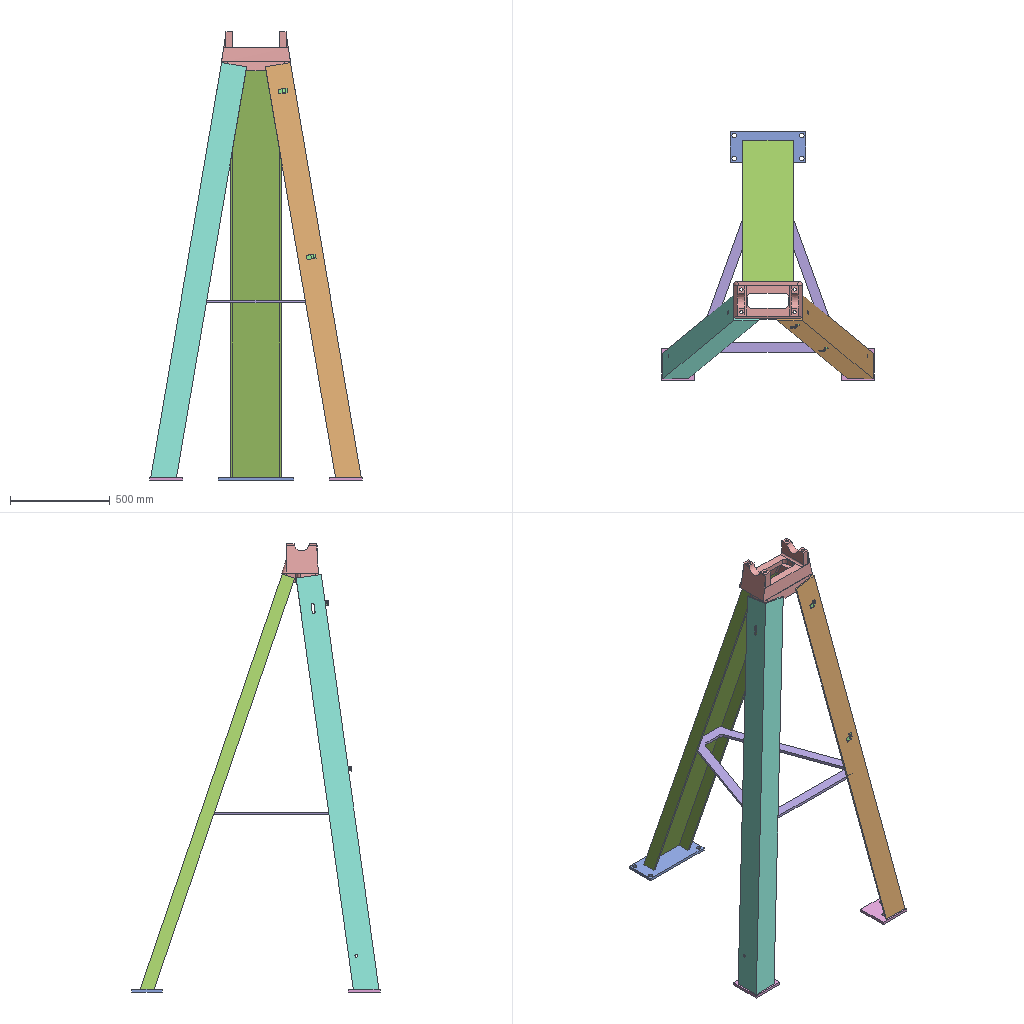Assembly | SolidWorks | 8 different items | 10 placed | box 1067 x 1244 x 2246 mm
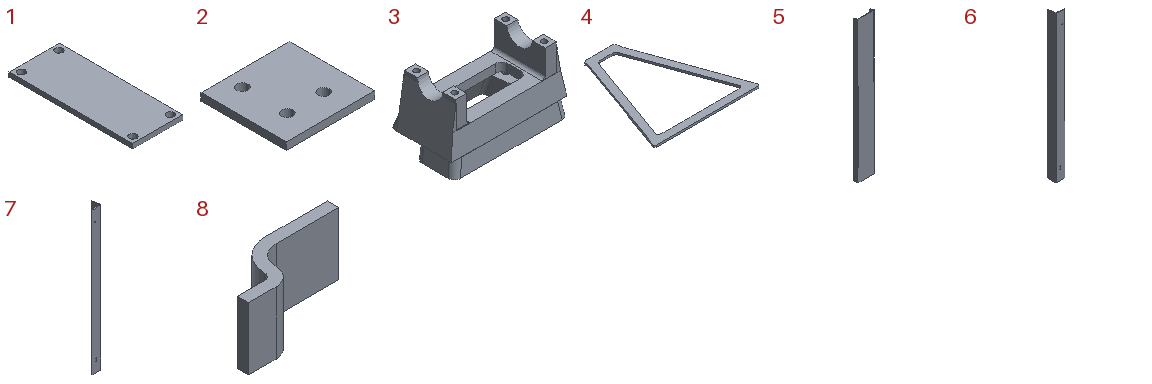Parts list (item | quantity | size | volume | features):
1 | x1 | 152.4 x 377.95 x 14 mm | 784620 mm3 | features Extrusion 1
2 | x2 | 166.35 x 160 x 14 mm | 358558 mm3 | features Extrusion 1
3 | x1 | 345.24 x 198.628 x 194.462 mm | 2581916 mm3 | features ICE 7, Fillet 5, Blend 2, Shell 1
4 | x1 | 733.425 x 755.65 x 14 mm | 1663233 mm3 | features Extrusion 1
5 | x1 | 254 x 66.04 x 2199 mm | 6305556 mm3 | features Extrusion 1, ICE 1
6 | x1 | 127 x 127 x 2128 mm | 4129005 mm3 | features ICE 2, Extrusion 1
7 | x1 | 127 x 127 x 2128 mm | 4129005 mm3 | features ICE 2, Extrusion 1
8 | x2 | 45.542 x 17.392 x 22.352 mm | 4755 mm3 | features Extrusion 1
Mates (type | each side: item.copy, entity, surface, feature):
Coincident | 3.1 plane | assembly plane
DistanceDim | assembly plane | 3.1 face plane Boss-Extrude2
Symmetric | 3.1 face plane Boss-Extrude2 | 3.1 face plane Boss-Extrude2 | assembly plane
DistanceDim | assembly plane | 1.1 face plane Boss-Extrude1
Coincident | 1.1 plane | assembly plane
DistanceDim | 1.1 face plane Boss-Extrude1 | assembly plane
Coincident | 5.1 plane | assembly plane
Coincident | 1.1 face plane Boss-Extrude1 | 5.1 face plane Cut-Extrude1
Coincident | 3.1 face plane Loft1 | 5.1 edge
Coincident | 1.1 face plane Boss-Extrude1 | 2.1 face plane Boss-Extrude1
DistanceDim | 2.1 face plane Boss-Extrude1 | 1.1 face plane Boss-Extrude1
Coincident | 3.1 face plane Loft1 | 7.1 edge
Coincident | 3.1 face plane Loft1 | 7.1 vertex
Coincident | 2.1 face plane Boss-Extrude1 | 6.1 vertex
DistanceDim | 6.1 vertex | 2.1 face plane Boss-Extrude1 | 2 times
Coincident | 3.1 face plane Loft1 | 6.1 edge
Coincident | 3.1 face plane Loft1 | 6.1 vertex
DistanceDim | 4.1 face plane Boss-Extrude1 | 2.1 face plane Boss-Extrude1
Coincident | 4.1 plane | assembly plane
Coincident | 5.1 face plane Boss-Extrude1 | 4.1 edge
Coincident | 7.1 face plane Boss-Extrude1 | 8.1 face plane Boss-Extrude1
Parallel | 7.1 face plane Boss-Extrude1 | 8.1 face plane Boss-Extrude1
DistanceDim | 8.1 face plane Boss-Extrude1 | 7.1 face plane Boss-Extrude1
Coincident | 2.1 face plane Boss-Extrude1 | 2.2 face plane Boss-Extrude1 | 2 times
Symmetric | 2.1 face plane Boss-Extrude1 | 2.2 face plane Boss-Extrude1 | assembly plane
Coincident | 2.2 face plane Boss-Extrude1 | 7.1 vertex
DistanceDim | 7.1 vertex | 2.2 face plane Boss-Extrude1 | 2 times
DistanceDim | 2.2 edge | 8.1 vertex
DistanceDim | 2.1 face plane Boss-Extrude1 | 2.2 face plane Boss-Extrude1